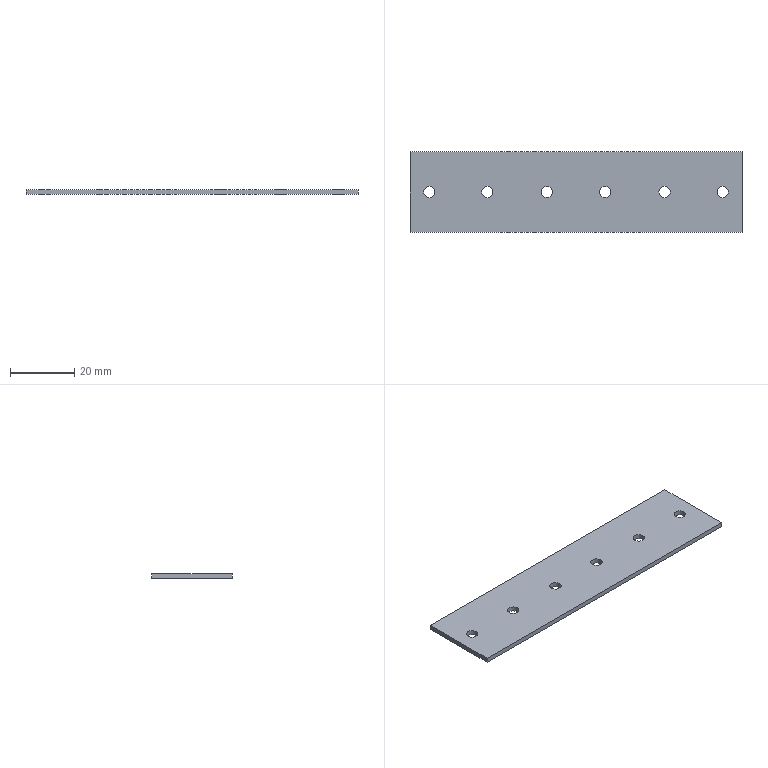Part | STEP file | FHD-021-008-03 fixing plate | 1 solid | 12 faces | box 103 x 25 x 1.5 mm | volume 3776 mm3 | plane 6 | cylinder 6 | commonest cylinder face diameters 3.5 x6
STEP:
#1=CARTESIAN_POINT('',(0.,0.,0.));
#2=DIRECTION('',(0.,0.,1.));
#3=DIRECTION('',(1.,0.,0.));
#4=AXIS2_PLACEMENT_3D('',#1,#2,#3);
#5=CARTESIAN_POINT('',(-51.5,-12.5,-1.5));
#6=VERTEX_POINT('',#5);
#7=CARTESIAN_POINT('',(-51.5,12.5,-1.5));
#8=VERTEX_POINT('',#7);
#9=CARTESIAN_POINT('',(-51.5,0.,-1.5));
#10=DIRECTION('',(0.,1.,0.));
#11=VECTOR('',#10,1.);
#12=LINE('',#9,#11);
#13=CARTESIAN_POINT('',(0.,0.,-1.5));
#14=DIRECTION('',(0.,0.,-1.));
#15=DIRECTION('',(-1.,0.,0.));
#16=AXIS2_PLACEMENT_3D('',#13,#14,#15);
#17=PLANE('',#16);
#18=CARTESIAN_POINT('',(51.5,0.));
#19=DIRECTION('',(0.,1.));
#20=VECTOR('',#19,1.);
#21=LINE('',#18,#20);
#22=(GEOMETRIC_REPRESENTATION_CONTEXT(2)PARAMETRIC_REPRESENTATION_CONTEXT()REPRESENTATION_CONTEXT('',''));
#23=DEFINITIONAL_REPRESENTATION('',(#21),#22);
#24=PCURVE('',#17,#23);
#25=CARTESIAN_POINT('',(-51.5,-12.5,-1.5));
#26=DIRECTION('',(-1.,0.,0.));
#27=DIRECTION('',(0.,0.,1.));
#28=AXIS2_PLACEMENT_3D('',#25,#26,#27);
#29=PLANE('',#28);
#30=CARTESIAN_POINT('',(0.,12.5));
#31=DIRECTION('',(0.,1.));
#32=VECTOR('',#31,1.);
#33=LINE('',#30,#32);
#34=(GEOMETRIC_REPRESENTATION_CONTEXT(2)PARAMETRIC_REPRESENTATION_CONTEXT()REPRESENTATION_CONTEXT('',''));
#35=DEFINITIONAL_REPRESENTATION('',(#33),#34);
#36=PCURVE('',#29,#35);
#37=SURFACE_CURVE('',#12,(#24,#36),.PCURVE_S1.);
#38=EDGE_CURVE('',#6,#8,#37,.T.);
#39=ORIENTED_EDGE('',*,*,#38,.T.);
#40=CARTESIAN_POINT('',(51.5,12.5,-1.5));
#41=VERTEX_POINT('',#40);
#42=CARTESIAN_POINT('',(0.,12.5,-1.5));
#43=DIRECTION('',(1.,0.,0.));
#44=VECTOR('',#43,1.);
#45=LINE('',#42,#44);
#46=CARTESIAN_POINT('',(0.,12.5));
#47=DIRECTION('',(-1.,0.));
#48=VECTOR('',#47,1.);
#49=LINE('',#46,#48);
#50=(GEOMETRIC_REPRESENTATION_CONTEXT(2)PARAMETRIC_REPRESENTATION_CONTEXT()REPRESENTATION_CONTEXT('',''));
#51=DEFINITIONAL_REPRESENTATION('',(#49),#50);
#52=PCURVE('',#17,#51);
#53=CARTESIAN_POINT('',(-51.5,12.5,-1.5));
#54=DIRECTION('',(0.,1.,0.));
#55=DIRECTION('',(0.,0.,1.));
#56=AXIS2_PLACEMENT_3D('',#53,#54,#55);
#57=PLANE('',#56);
#58=CARTESIAN_POINT('',(0.,51.5));
#59=DIRECTION('',(0.,1.));
#60=VECTOR('',#59,1.);
#61=LINE('',#58,#60);
#62=(GEOMETRIC_REPRESENTATION_CONTEXT(2)PARAMETRIC_REPRESENTATION_CONTEXT()REPRESENTATION_CONTEXT('',''));
#63=DEFINITIONAL_REPRESENTATION('',(#61),#62);
#64=PCURVE('',#57,#63);
#65=SURFACE_CURVE('',#45,(#52,#64),.PCURVE_S1.);
#66=EDGE_CURVE('',#8,#41,#65,.T.);
#67=ORIENTED_EDGE('',*,*,#66,.T.);
#68=CARTESIAN_POINT('',(51.5,-12.5,-1.5));
#69=VERTEX_POINT('',#68);
#70=CARTESIAN_POINT('',(51.5,0.,-1.5));
#71=DIRECTION('',(0.,-1.,0.));
#72=VECTOR('',#71,1.);
#73=LINE('',#70,#72);
#74=CARTESIAN_POINT('',(-51.5,0.));
#75=DIRECTION('',(0.,-1.));
#76=VECTOR('',#75,1.);
#77=LINE('',#74,#76);
#78=(GEOMETRIC_REPRESENTATION_CONTEXT(2)PARAMETRIC_REPRESENTATION_CONTEXT()REPRESENTATION_CONTEXT('',''));
#79=DEFINITIONAL_REPRESENTATION('',(#77),#78);
#80=PCURVE('',#17,#79);
#81=CARTESIAN_POINT('',(51.5,-12.5,-1.5));
#82=DIRECTION('',(1.,0.,0.));
#83=DIRECTION('',(0.,0.,-1.));
#84=AXIS2_PLACEMENT_3D('',#81,#82,#83);
#85=PLANE('',#84);
#86=CARTESIAN_POINT('',(0.,12.5));
#87=DIRECTION('',(0.,-1.));
#88=VECTOR('',#87,1.);
#89=LINE('',#86,#88);
#90=(GEOMETRIC_REPRESENTATION_CONTEXT(2)PARAMETRIC_REPRESENTATION_CONTEXT()REPRESENTATION_CONTEXT('',''));
#91=DEFINITIONAL_REPRESENTATION('',(#89),#90);
#92=PCURVE('',#85,#91);
#93=SURFACE_CURVE('',#73,(#80,#92),.PCURVE_S1.);
#94=EDGE_CURVE('',#41,#69,#93,.T.);
#95=ORIENTED_EDGE('',*,*,#94,.T.);
#96=CARTESIAN_POINT('',(0.,-12.5,-1.5));
#97=DIRECTION('',(-1.,0.,0.));
#98=VECTOR('',#97,1.);
#99=LINE('',#96,#98);
#100=CARTESIAN_POINT('',(0.,-12.5));
#101=DIRECTION('',(1.,0.));
#102=VECTOR('',#101,1.);
#103=LINE('',#100,#102);
#104=(GEOMETRIC_REPRESENTATION_CONTEXT(2)PARAMETRIC_REPRESENTATION_CONTEXT()REPRESENTATION_CONTEXT('',''));
#105=DEFINITIONAL_REPRESENTATION('',(#103),#104);
#106=PCURVE('',#17,#105);
#107=CARTESIAN_POINT('',(-51.5,-12.5,-1.5));
#108=DIRECTION('',(0.,-1.,0.));
#109=DIRECTION('',(0.,0.,-1.));
#110=AXIS2_PLACEMENT_3D('',#107,#108,#109);
#111=PLANE('',#110);
#112=CARTESIAN_POINT('',(0.,51.5));
#113=DIRECTION('',(0.,-1.));
#114=VECTOR('',#113,1.);
#115=LINE('',#112,#114);
#116=(GEOMETRIC_REPRESENTATION_CONTEXT(2)PARAMETRIC_REPRESENTATION_CONTEXT()REPRESENTATION_CONTEXT('',''));
#117=DEFINITIONAL_REPRESENTATION('',(#115),#116);
#118=PCURVE('',#111,#117);
#119=SURFACE_CURVE('',#99,(#106,#118),.PCURVE_S1.);
#120=EDGE_CURVE('',#69,#6,#119,.T.);
#121=ORIENTED_EDGE('',*,*,#120,.T.);
#122=EDGE_LOOP('',(#39,#67,#95,#121));
#123=FACE_BOUND('',#122,.T.);
#124=CARTESIAN_POINT('',(47.25,0.,-1.5));
#125=VERTEX_POINT('',#124);
#126=CARTESIAN_POINT('',(45.5,0.,-1.5));
#127=DIRECTION('',(0.,0.,1.));
#128=DIRECTION('',(1.,0.,0.));
#129=AXIS2_PLACEMENT_3D('',#126,#127,#128);
#130=CIRCLE('',#129,1.75);
#131=CARTESIAN_POINT('',(-47.25,0.));
#132=CARTESIAN_POINT('',(-47.25,3.031));
#133=CARTESIAN_POINT('',(-44.625,1.516));
#134=CARTESIAN_POINT('',(-42.,0.));
#135=CARTESIAN_POINT('',(-44.625,-1.516));
#136=CARTESIAN_POINT('',(-47.25,-3.031));
#137=CARTESIAN_POINT('',(-47.25,0.));
#138=(BOUNDED_CURVE()B_SPLINE_CURVE(2,(#131,#132,#133,#134,#135,#136,#137),.UNSPECIFIED.,.T.,.F.)B_SPLINE_CURVE_WITH_KNOTS((1,2,2,2,2,1),(-2.094,0.,2.094,4.189,6.283,8.378),.UNSPECIFIED.)CURVE()GEOMETRIC_REPRESENTATION_ITEM()RATIONAL_B_SPLINE_CURVE((1.,0.5,1.,0.5,1.,0.5,1.))REPRESENTATION_ITEM(''));
#139=(GEOMETRIC_REPRESENTATION_CONTEXT(2)PARAMETRIC_REPRESENTATION_CONTEXT()REPRESENTATION_CONTEXT('',''));
#140=DEFINITIONAL_REPRESENTATION('',(#138),#139);
#141=PCURVE('',#17,#140);
#142=CARTESIAN_POINT('',(45.5,0.,-10.));
#143=DIRECTION('',(0.,0.,1.));
#144=DIRECTION('',(1.,0.,0.));
#145=AXIS2_PLACEMENT_3D('',#142,#143,#144);
#146=CYLINDRICAL_SURFACE('',#145,1.75);
#147=CARTESIAN_POINT('',(0.,8.5));
#148=DIRECTION('',(1.,0.));
#149=VECTOR('',#148,1.);
#150=LINE('',#147,#149);
#151=(GEOMETRIC_REPRESENTATION_CONTEXT(2)PARAMETRIC_REPRESENTATION_CONTEXT()REPRESENTATION_CONTEXT('',''));
#152=DEFINITIONAL_REPRESENTATION('',(#150),#151);
#153=PCURVE('',#146,#152);
#154=SURFACE_CURVE('',#130,(#141,#153),.PCURVE_S1.);
#155=EDGE_CURVE('',#125,#125,#154,.T.);
#156=ORIENTED_EDGE('',*,*,#155,.T.);
#157=EDGE_LOOP('',(#156));
#158=FACE_BOUND('',#157,.T.);
#159=CARTESIAN_POINT('',(-43.75,0.,-1.5));
#160=VERTEX_POINT('',#159);
#161=CARTESIAN_POINT('',(-45.5,0.,-1.5));
#162=DIRECTION('',(0.,0.,1.));
#163=DIRECTION('',(1.,0.,0.));
#164=AXIS2_PLACEMENT_3D('',#161,#162,#163);
#165=CIRCLE('',#164,1.75);
#166=CARTESIAN_POINT('',(43.75,0.));
#167=CARTESIAN_POINT('',(43.75,3.031));
#168=CARTESIAN_POINT('',(46.375,1.516));
#169=CARTESIAN_POINT('',(49.,0.));
#170=CARTESIAN_POINT('',(46.375,-1.516));
#171=CARTESIAN_POINT('',(43.75,-3.031));
#172=CARTESIAN_POINT('',(43.75,0.));
#173=(BOUNDED_CURVE()B_SPLINE_CURVE(2,(#166,#167,#168,#169,#170,#171,#172),.UNSPECIFIED.,.T.,.F.)B_SPLINE_CURVE_WITH_KNOTS((1,2,2,2,2,1),(-2.094,0.,2.094,4.189,6.283,8.378),.UNSPECIFIED.)CURVE()GEOMETRIC_REPRESENTATION_ITEM()RATIONAL_B_SPLINE_CURVE((1.,0.5,1.,0.5,1.,0.5,1.))REPRESENTATION_ITEM(''));
#174=(GEOMETRIC_REPRESENTATION_CONTEXT(2)PARAMETRIC_REPRESENTATION_CONTEXT()REPRESENTATION_CONTEXT('',''));
#175=DEFINITIONAL_REPRESENTATION('',(#173),#174);
#176=PCURVE('',#17,#175);
#177=CARTESIAN_POINT('',(-45.5,0.,-10.));
#178=DIRECTION('',(0.,0.,1.));
#179=DIRECTION('',(1.,0.,0.));
#180=AXIS2_PLACEMENT_3D('',#177,#178,#179);
#181=CYLINDRICAL_SURFACE('',#180,1.75);
#182=CARTESIAN_POINT('',(0.,8.5));
#183=DIRECTION('',(1.,0.));
#184=VECTOR('',#183,1.);
#185=LINE('',#182,#184);
#186=(GEOMETRIC_REPRESENTATION_CONTEXT(2)PARAMETRIC_REPRESENTATION_CONTEXT()REPRESENTATION_CONTEXT('',''));
#187=DEFINITIONAL_REPRESENTATION('',(#185),#186);
#188=PCURVE('',#181,#187);
#189=SURFACE_CURVE('',#165,(#176,#188),.PCURVE_S1.);
#190=EDGE_CURVE('',#160,#160,#189,.T.);
#191=ORIENTED_EDGE('',*,*,#190,.T.);
#192=EDGE_LOOP('',(#191));
#193=FACE_BOUND('',#192,.T.);
#194=CARTESIAN_POINT('',(29.25,0.,-1.5));
#195=VERTEX_POINT('',#194);
#196=CARTESIAN_POINT('',(27.5,0.,-1.5));
#197=DIRECTION('',(0.,0.,1.));
#198=DIRECTION('',(1.,0.,0.));
#199=AXIS2_PLACEMENT_3D('',#196,#197,#198);
#200=CIRCLE('',#199,1.75);
#201=CARTESIAN_POINT('',(-29.25,0.));
#202=CARTESIAN_POINT('',(-29.25,3.031));
#203=CARTESIAN_POINT('',(-26.625,1.516));
#204=CARTESIAN_POINT('',(-24.,0.));
#205=CARTESIAN_POINT('',(-26.625,-1.516));
#206=CARTESIAN_POINT('',(-29.25,-3.031));
#207=CARTESIAN_POINT('',(-29.25,0.));
#208=(BOUNDED_CURVE()B_SPLINE_CURVE(2,(#201,#202,#203,#204,#205,#206,#207),.UNSPECIFIED.,.T.,.F.)B_SPLINE_CURVE_WITH_KNOTS((1,2,2,2,2,1),(-2.094,0.,2.094,4.189,6.283,8.378),.UNSPECIFIED.)CURVE()GEOMETRIC_REPRESENTATION_ITEM()RATIONAL_B_SPLINE_CURVE((1.,0.5,1.,0.5,1.,0.5,1.))REPRESENTATION_ITEM(''));
#209=(GEOMETRIC_REPRESENTATION_CONTEXT(2)PARAMETRIC_REPRESENTATION_CONTEXT()REPRESENTATION_CONTEXT('',''));
#210=DEFINITIONAL_REPRESENTATION('',(#208),#209);
#211=PCURVE('',#17,#210);
#212=CARTESIAN_POINT('',(27.5,0.,-10.));
#213=DIRECTION('',(0.,0.,1.));
#214=DIRECTION('',(1.,0.,0.));
#215=AXIS2_PLACEMENT_3D('',#212,#213,#214);
#216=CYLINDRICAL_SURFACE('',#215,1.75);
#217=CARTESIAN_POINT('',(0.,8.5));
#218=DIRECTION('',(1.,0.));
#219=VECTOR('',#218,1.);
#220=LINE('',#217,#219);
#221=(GEOMETRIC_REPRESENTATION_CONTEXT(2)PARAMETRIC_REPRESENTATION_CONTEXT()REPRESENTATION_CONTEXT('',''));
#222=DEFINITIONAL_REPRESENTATION('',(#220),#221);
#223=PCURVE('',#216,#222);
#224=SURFACE_CURVE('',#200,(#211,#223),.PCURVE_S1.);
#225=EDGE_CURVE('',#195,#195,#224,.T.);
#226=ORIENTED_EDGE('',*,*,#225,.T.);
#227=EDGE_LOOP('',(#226));
#228=FACE_BOUND('',#227,.T.);
#229=CARTESIAN_POINT('',(10.75,0.,-1.5));
#230=VERTEX_POINT('',#229);
#231=CARTESIAN_POINT('',(9.,0.,-1.5));
#232=DIRECTION('',(0.,0.,1.));
#233=DIRECTION('',(1.,0.,0.));
#234=AXIS2_PLACEMENT_3D('',#231,#232,#233);
#235=CIRCLE('',#234,1.75);
#236=CARTESIAN_POINT('',(-10.75,0.));
#237=CARTESIAN_POINT('',(-10.75,3.031));
#238=CARTESIAN_POINT('',(-8.125,1.516));
#239=CARTESIAN_POINT('',(-5.5,0.));
#240=CARTESIAN_POINT('',(-8.125,-1.516));
#241=CARTESIAN_POINT('',(-10.75,-3.031));
#242=CARTESIAN_POINT('',(-10.75,0.));
#243=(BOUNDED_CURVE()B_SPLINE_CURVE(2,(#236,#237,#238,#239,#240,#241,#242),.UNSPECIFIED.,.T.,.F.)B_SPLINE_CURVE_WITH_KNOTS((1,2,2,2,2,1),(-2.094,0.,2.094,4.189,6.283,8.378),.UNSPECIFIED.)CURVE()GEOMETRIC_REPRESENTATION_ITEM()RATIONAL_B_SPLINE_CURVE((1.,0.5,1.,0.5,1.,0.5,1.))REPRESENTATION_ITEM(''));
#244=(GEOMETRIC_REPRESENTATION_CONTEXT(2)PARAMETRIC_REPRESENTATION_CONTEXT()REPRESENTATION_CONTEXT('',''));
#245=DEFINITIONAL_REPRESENTATION('',(#243),#244);
#246=PCURVE('',#17,#245);
#247=CARTESIAN_POINT('',(9.,0.,-10.));
#248=DIRECTION('',(0.,0.,1.));
#249=DIRECTION('',(1.,0.,0.));
#250=AXIS2_PLACEMENT_3D('',#247,#248,#249);
#251=CYLINDRICAL_SURFACE('',#250,1.75);
#252=CARTESIAN_POINT('',(0.,8.5));
#253=DIRECTION('',(1.,0.));
#254=VECTOR('',#253,1.);
#255=LINE('',#252,#254);
#256=(GEOMETRIC_REPRESENTATION_CONTEXT(2)PARAMETRIC_REPRESENTATION_CONTEXT()REPRESENTATION_CONTEXT('',''));
#257=DEFINITIONAL_REPRESENTATION('',(#255),#256);
#258=PCURVE('',#251,#257);
#259=SURFACE_CURVE('',#235,(#246,#258),.PCURVE_S1.);
#260=EDGE_CURVE('',#230,#230,#259,.T.);
#261=ORIENTED_EDGE('',*,*,#260,.T.);
#262=EDGE_LOOP('',(#261));
#263=FACE_BOUND('',#262,.T.);
#264=CARTESIAN_POINT('',(-7.25,0.,-1.5));
#265=VERTEX_POINT('',#264);
#266=CARTESIAN_POINT('',(-9.,0.,-1.5));
#267=DIRECTION('',(0.,0.,1.));
#268=DIRECTION('',(1.,0.,0.));
#269=AXIS2_PLACEMENT_3D('',#266,#267,#268);
#270=CIRCLE('',#269,1.75);
#271=CARTESIAN_POINT('',(7.25,0.));
#272=CARTESIAN_POINT('',(7.25,3.031));
#273=CARTESIAN_POINT('',(9.875,1.516));
#274=CARTESIAN_POINT('',(12.5,0.));
#275=CARTESIAN_POINT('',(9.875,-1.516));
#276=CARTESIAN_POINT('',(7.25,-3.031));
#277=CARTESIAN_POINT('',(7.25,0.));
#278=(BOUNDED_CURVE()B_SPLINE_CURVE(2,(#271,#272,#273,#274,#275,#276,#277),.UNSPECIFIED.,.T.,.F.)B_SPLINE_CURVE_WITH_KNOTS((1,2,2,2,2,1),(-2.094,0.,2.094,4.189,6.283,8.378),.UNSPECIFIED.)CURVE()GEOMETRIC_REPRESENTATION_ITEM()RATIONAL_B_SPLINE_CURVE((1.,0.5,1.,0.5,1.,0.5,1.))REPRESENTATION_ITEM(''));
#279=(GEOMETRIC_REPRESENTATION_CONTEXT(2)PARAMETRIC_REPRESENTATION_CONTEXT()REPRESENTATION_CONTEXT('',''));
#280=DEFINITIONAL_REPRESENTATION('',(#278),#279);
#281=PCURVE('',#17,#280);
#282=CARTESIAN_POINT('',(-9.,0.,-10.));
#283=DIRECTION('',(0.,0.,1.));
#284=DIRECTION('',(1.,0.,0.));
#285=AXIS2_PLACEMENT_3D('',#282,#283,#284);
#286=CYLINDRICAL_SURFACE('',#285,1.75);
#287=CARTESIAN_POINT('',(0.,8.5));
#288=DIRECTION('',(1.,0.));
#289=VECTOR('',#288,1.);
#290=LINE('',#287,#289);
#291=(GEOMETRIC_REPRESENTATION_CONTEXT(2)PARAMETRIC_REPRESENTATION_CONTEXT()REPRESENTATION_CONTEXT('',''));
#292=DEFINITIONAL_REPRESENTATION('',(#290),#291);
#293=PCURVE('',#286,#292);
#294=SURFACE_CURVE('',#270,(#281,#293),.PCURVE_S1.);
#295=EDGE_CURVE('',#265,#265,#294,.T.);
#296=ORIENTED_EDGE('',*,*,#295,.T.);
#297=EDGE_LOOP('',(#296));
#298=FACE_BOUND('',#297,.T.);
#299=CARTESIAN_POINT('',(-25.75,0.,-1.5));
#300=VERTEX_POINT('',#299);
#301=CARTESIAN_POINT('',(-27.5,0.,-1.5));
#302=DIRECTION('',(0.,0.,1.));
#303=DIRECTION('',(1.,0.,0.));
#304=AXIS2_PLACEMENT_3D('',#301,#302,#303);
#305=CIRCLE('',#304,1.75);
#306=CARTESIAN_POINT('',(25.75,0.));
#307=CARTESIAN_POINT('',(25.75,3.031));
#308=CARTESIAN_POINT('',(28.375,1.516));
#309=CARTESIAN_POINT('',(31.,0.));
#310=CARTESIAN_POINT('',(28.375,-1.516));
#311=CARTESIAN_POINT('',(25.75,-3.031));
#312=CARTESIAN_POINT('',(25.75,0.));
#313=(BOUNDED_CURVE()B_SPLINE_CURVE(2,(#306,#307,#308,#309,#310,#311,#312),.UNSPECIFIED.,.T.,.F.)B_SPLINE_CURVE_WITH_KNOTS((1,2,2,2,2,1),(-2.094,0.,2.094,4.189,6.283,8.378),.UNSPECIFIED.)CURVE()GEOMETRIC_REPRESENTATION_ITEM()RATIONAL_B_SPLINE_CURVE((1.,0.5,1.,0.5,1.,0.5,1.))REPRESENTATION_ITEM(''));
#314=(GEOMETRIC_REPRESENTATION_CONTEXT(2)PARAMETRIC_REPRESENTATION_CONTEXT()REPRESENTATION_CONTEXT('',''));
#315=DEFINITIONAL_REPRESENTATION('',(#313),#314);
#316=PCURVE('',#17,#315);
#317=CARTESIAN_POINT('',(-27.5,0.,-10.));
#318=DIRECTION('',(0.,0.,1.));
#319=DIRECTION('',(1.,0.,0.));
#320=AXIS2_PLACEMENT_3D('',#317,#318,#319);
#321=CYLINDRICAL_SURFACE('',#320,1.75);
#322=CARTESIAN_POINT('',(0.,8.5));
#323=DIRECTION('',(1.,0.));
#324=VECTOR('',#323,1.);
#325=LINE('',#322,#324);
#326=(GEOMETRIC_REPRESENTATION_CONTEXT(2)PARAMETRIC_REPRESENTATION_CONTEXT()REPRESENTATION_CONTEXT('',''));
#327=DEFINITIONAL_REPRESENTATION('',(#325),#326);
#328=PCURVE('',#321,#327);
#329=SURFACE_CURVE('',#305,(#316,#328),.PCURVE_S1.);
#330=EDGE_CURVE('',#300,#300,#329,.T.);
#331=ORIENTED_EDGE('',*,*,#330,.T.);
#332=EDGE_LOOP('',(#331));
#333=FACE_BOUND('',#332,.T.);
#334=ADVANCED_FACE('',(#123,#158,#193,#228,#263,#298,#333),#17,.T.);
#335=ORIENTED_EDGE('',*,*,#66,.F.);
#336=CARTESIAN_POINT('',(-51.5,12.5,0.));
#337=VERTEX_POINT('',#336);
#338=CARTESIAN_POINT('',(-51.5,12.5,-1.5));
#339=DIRECTION('',(0.,0.,1.));
#340=VECTOR('',#339,1.);
#341=LINE('',#338,#340);
#342=CARTESIAN_POINT('',(0.,0.));
#343=DIRECTION('',(1.,0.));
#344=VECTOR('',#343,1.);
#345=LINE('',#342,#344);
#346=(GEOMETRIC_REPRESENTATION_CONTEXT(2)PARAMETRIC_REPRESENTATION_CONTEXT()REPRESENTATION_CONTEXT('',''));
#347=DEFINITIONAL_REPRESENTATION('',(#345),#346);
#348=PCURVE('',#57,#347);
#349=CARTESIAN_POINT('',(0.,25.));
#350=DIRECTION('',(1.,0.));
#351=VECTOR('',#350,1.);
#352=LINE('',#349,#351);
#353=(GEOMETRIC_REPRESENTATION_CONTEXT(2)PARAMETRIC_REPRESENTATION_CONTEXT()REPRESENTATION_CONTEXT('',''));
#354=DEFINITIONAL_REPRESENTATION('',(#352),#353);
#355=PCURVE('',#29,#354);
#356=SURFACE_CURVE('',#341,(#348,#355),.PCURVE_S1.);
#357=EDGE_CURVE('',#8,#337,#356,.T.);
#358=ORIENTED_EDGE('',*,*,#357,.T.);
#359=CARTESIAN_POINT('',(51.5,12.5,0.));
#360=VERTEX_POINT('',#359);
#361=CARTESIAN_POINT('',(-51.5,12.5,0.));
#362=DIRECTION('',(1.,0.,0.));
#363=VECTOR('',#362,1.);
#364=LINE('',#361,#363);
#365=CARTESIAN_POINT('',(1.5,0.));
#366=DIRECTION('',(0.,1.));
#367=VECTOR('',#366,1.);
#368=LINE('',#365,#367);
#369=(GEOMETRIC_REPRESENTATION_CONTEXT(2)PARAMETRIC_REPRESENTATION_CONTEXT()REPRESENTATION_CONTEXT('',''));
#370=DEFINITIONAL_REPRESENTATION('',(#368),#369);
#371=PCURVE('',#57,#370);
#372=CARTESIAN_POINT('',(0.,0.,0.));
#373=DIRECTION('',(0.,0.,-1.));
#374=DIRECTION('',(-1.,0.,0.));
#375=AXIS2_PLACEMENT_3D('',#372,#373,#374);
#376=PLANE('',#375);
#377=CARTESIAN_POINT('',(51.5,12.5));
#378=DIRECTION('',(-1.,0.));
#379=VECTOR('',#378,1.);
#380=LINE('',#377,#379);
#381=(GEOMETRIC_REPRESENTATION_CONTEXT(2)PARAMETRIC_REPRESENTATION_CONTEXT()REPRESENTATION_CONTEXT('',''));
#382=DEFINITIONAL_REPRESENTATION('',(#380),#381);
#383=PCURVE('',#376,#382);
#384=SURFACE_CURVE('',#364,(#371,#383),.PCURVE_S1.);
#385=EDGE_CURVE('',#337,#360,#384,.T.);
#386=ORIENTED_EDGE('',*,*,#385,.T.);
#387=CARTESIAN_POINT('',(51.5,12.5,-1.5));
#388=DIRECTION('',(0.,0.,-1.));
#389=VECTOR('',#388,1.);
#390=LINE('',#387,#389);
#391=CARTESIAN_POINT('',(0.,103.));
#392=DIRECTION('',(-1.,0.));
#393=VECTOR('',#392,1.);
#394=LINE('',#391,#393);
#395=(GEOMETRIC_REPRESENTATION_CONTEXT(2)PARAMETRIC_REPRESENTATION_CONTEXT()REPRESENTATION_CONTEXT('',''));
#396=DEFINITIONAL_REPRESENTATION('',(#394),#395);
#397=PCURVE('',#57,#396);
#398=CARTESIAN_POINT('',(0.,25.));
#399=DIRECTION('',(1.,0.));
#400=VECTOR('',#399,1.);
#401=LINE('',#398,#400);
#402=(GEOMETRIC_REPRESENTATION_CONTEXT(2)PARAMETRIC_REPRESENTATION_CONTEXT()REPRESENTATION_CONTEXT('',''));
#403=DEFINITIONAL_REPRESENTATION('',(#401),#402);
#404=PCURVE('',#85,#403);
#405=SURFACE_CURVE('',#390,(#397,#404),.PCURVE_S1.);
#406=EDGE_CURVE('',#360,#41,#405,.T.);
#407=ORIENTED_EDGE('',*,*,#406,.T.);
#408=EDGE_LOOP('',(#335,#358,#386,#407));
#409=FACE_BOUND('',#408,.T.);
#410=ADVANCED_FACE('',(#409),#57,.T.);
#411=ORIENTED_EDGE('',*,*,#38,.F.);
#412=CARTESIAN_POINT('',(-51.5,-12.5,0.));
#413=VERTEX_POINT('',#412);
#414=CARTESIAN_POINT('',(-51.5,-12.5,-1.5));
#415=DIRECTION('',(0.,0.,1.));
#416=VECTOR('',#415,1.);
#417=LINE('',#414,#416);
#418=CARTESIAN_POINT('',(0.,0.));
#419=DIRECTION('',(1.,0.));
#420=VECTOR('',#419,1.);
#421=LINE('',#418,#420);
#422=(GEOMETRIC_REPRESENTATION_CONTEXT(2)PARAMETRIC_REPRESENTATION_CONTEXT()REPRESENTATION_CONTEXT('',''));
#423=DEFINITIONAL_REPRESENTATION('',(#421),#422);
#424=PCURVE('',#29,#423);
#425=CARTESIAN_POINT('',(0.,0.));
#426=DIRECTION('',(-1.,0.));
#427=VECTOR('',#426,1.);
#428=LINE('',#425,#427);
#429=(GEOMETRIC_REPRESENTATION_CONTEXT(2)PARAMETRIC_REPRESENTATION_CONTEXT()REPRESENTATION_CONTEXT('',''));
#430=DEFINITIONAL_REPRESENTATION('',(#428),#429);
#431=PCURVE('',#111,#430);
#432=SURFACE_CURVE('',#417,(#424,#431),.PCURVE_S1.);
#433=EDGE_CURVE('',#6,#413,#432,.T.);
#434=ORIENTED_EDGE('',*,*,#433,.T.);
#435=CARTESIAN_POINT('',(-51.5,-12.5,0.));
#436=DIRECTION('',(0.,1.,0.));
#437=VECTOR('',#436,1.);
#438=LINE('',#435,#437);
#439=CARTESIAN_POINT('',(1.5,0.));
#440=DIRECTION('',(0.,1.));
#441=VECTOR('',#440,1.);
#442=LINE('',#439,#441);
#443=(GEOMETRIC_REPRESENTATION_CONTEXT(2)PARAMETRIC_REPRESENTATION_CONTEXT()REPRESENTATION_CONTEXT('',''));
#444=DEFINITIONAL_REPRESENTATION('',(#442),#443);
#445=PCURVE('',#29,#444);
#446=CARTESIAN_POINT('',(51.5,-12.5));
#447=DIRECTION('',(0.,1.));
#448=VECTOR('',#447,1.);
#449=LINE('',#446,#448);
#450=(GEOMETRIC_REPRESENTATION_CONTEXT(2)PARAMETRIC_REPRESENTATION_CONTEXT()REPRESENTATION_CONTEXT('',''));
#451=DEFINITIONAL_REPRESENTATION('',(#449),#450);
#452=PCURVE('',#376,#451);
#453=SURFACE_CURVE('',#438,(#445,#452),.PCURVE_S1.);
#454=EDGE_CURVE('',#413,#337,#453,.T.);
#455=ORIENTED_EDGE('',*,*,#454,.T.);
#456=ORIENTED_EDGE('',*,*,#357,.F.);
#457=EDGE_LOOP('',(#411,#434,#455,#456));
#458=FACE_BOUND('',#457,.T.);
#459=ADVANCED_FACE('',(#458),#29,.T.);
#460=ORIENTED_EDGE('',*,*,#120,.F.);
#461=CARTESIAN_POINT('',(51.5,-12.5,0.));
#462=VERTEX_POINT('',#461);
#463=CARTESIAN_POINT('',(51.5,-12.5,-1.5));
#464=DIRECTION('',(0.,0.,1.));
#465=VECTOR('',#464,1.);
#466=LINE('',#463,#465);
#467=CARTESIAN_POINT('',(0.,103.));
#468=DIRECTION('',(-1.,0.));
#469=VECTOR('',#468,1.);
#470=LINE('',#467,#469);
#471=(GEOMETRIC_REPRESENTATION_CONTEXT(2)PARAMETRIC_REPRESENTATION_CONTEXT()REPRESENTATION_CONTEXT('',''));
#472=DEFINITIONAL_REPRESENTATION('',(#470),#471);
#473=PCURVE('',#111,#472);
#474=CARTESIAN_POINT('',(0.,0.));
#475=DIRECTION('',(-1.,0.));
#476=VECTOR('',#475,1.);
#477=LINE('',#474,#476);
#478=(GEOMETRIC_REPRESENTATION_CONTEXT(2)PARAMETRIC_REPRESENTATION_CONTEXT()REPRESENTATION_CONTEXT('',''));
#479=DEFINITIONAL_REPRESENTATION('',(#477),#478);
#480=PCURVE('',#85,#479);
#481=SURFACE_CURVE('',#466,(#473,#480),.PCURVE_S1.);
#482=EDGE_CURVE('',#69,#462,#481,.T.);
#483=ORIENTED_EDGE('',*,*,#482,.T.);
#484=CARTESIAN_POINT('',(-51.5,-12.5,0.));
#485=DIRECTION('',(-1.,0.,0.));
#486=VECTOR('',#485,1.);
#487=LINE('',#484,#486);
#488=CARTESIAN_POINT('',(-1.5,0.));
#489=DIRECTION('',(0.,-1.));
#490=VECTOR('',#489,1.);
#491=LINE('',#488,#490);
#492=(GEOMETRIC_REPRESENTATION_CONTEXT(2)PARAMETRIC_REPRESENTATION_CONTEXT()REPRESENTATION_CONTEXT('',''));
#493=DEFINITIONAL_REPRESENTATION('',(#491),#492);
#494=PCURVE('',#111,#493);
#495=CARTESIAN_POINT('',(51.5,-12.5));
#496=DIRECTION('',(1.,0.));
#497=VECTOR('',#496,1.);
#498=LINE('',#495,#497);
#499=(GEOMETRIC_REPRESENTATION_CONTEXT(2)PARAMETRIC_REPRESENTATION_CONTEXT()REPRESENTATION_CONTEXT('',''));
#500=DEFINITIONAL_REPRESENTATION('',(#498),#499);
#501=PCURVE('',#376,#500);
#502=SURFACE_CURVE('',#487,(#494,#501),.PCURVE_S1.);
#503=EDGE_CURVE('',#462,#413,#502,.T.);
#504=ORIENTED_EDGE('',*,*,#503,.T.);
#505=ORIENTED_EDGE('',*,*,#433,.F.);
#506=EDGE_LOOP('',(#460,#483,#504,#505));
#507=FACE_BOUND('',#506,.T.);
#508=ADVANCED_FACE('',(#507),#111,.T.);
#509=ORIENTED_EDGE('',*,*,#94,.F.);
#510=ORIENTED_EDGE('',*,*,#406,.F.);
#511=CARTESIAN_POINT('',(51.5,-12.5,0.));
#512=DIRECTION('',(0.,-1.,0.));
#513=VECTOR('',#512,1.);
#514=LINE('',#511,#513);
#515=CARTESIAN_POINT('',(-1.5,0.));
#516=DIRECTION('',(0.,-1.));
#517=VECTOR('',#516,1.);
#518=LINE('',#515,#517);
#519=(GEOMETRIC_REPRESENTATION_CONTEXT(2)PARAMETRIC_REPRESENTATION_CONTEXT()REPRESENTATION_CONTEXT('',''));
#520=DEFINITIONAL_REPRESENTATION('',(#518),#519);
#521=PCURVE('',#85,#520);
#522=CARTESIAN_POINT('',(-51.5,-12.5));
#523=DIRECTION('',(0.,-1.));
#524=VECTOR('',#523,1.);
#525=LINE('',#522,#524);
#526=(GEOMETRIC_REPRESENTATION_CONTEXT(2)PARAMETRIC_REPRESENTATION_CONTEXT()REPRESENTATION_CONTEXT('',''));
#527=DEFINITIONAL_REPRESENTATION('',(#525),#526);
#528=PCURVE('',#376,#527);
#529=SURFACE_CURVE('',#514,(#521,#528),.PCURVE_S1.);
#530=EDGE_CURVE('',#360,#462,#529,.T.);
#531=ORIENTED_EDGE('',*,*,#530,.T.);
#532=ORIENTED_EDGE('',*,*,#482,.F.);
#533=EDGE_LOOP('',(#509,#510,#531,#532));
#534=FACE_BOUND('',#533,.T.);
#535=ADVANCED_FACE('',(#534),#85,.T.);
#536=ORIENTED_EDGE('',*,*,#155,.T.);
#537=CARTESIAN_POINT('',(47.25,0.,0.));
#538=VERTEX_POINT('',#537);
#539=CARTESIAN_POINT('',(47.25,0.,-1.5));
#540=CARTESIAN_POINT('',(47.25,0.,0.));
#541=B_SPLINE_CURVE_WITH_KNOTS('',1,(#539,#540),.UNSPECIFIED.,.F.,.F.,(2,2),(8.5,10.),.PIECEWISE_BEZIER_KNOTS.);
#542=CARTESIAN_POINT('',(6.283,0.));
#543=DIRECTION('',(0.,1.));
#544=VECTOR('',#543,1.);
#545=LINE('',#542,#544);
#546=(GEOMETRIC_REPRESENTATION_CONTEXT(2)PARAMETRIC_REPRESENTATION_CONTEXT()REPRESENTATION_CONTEXT('',''));
#547=DEFINITIONAL_REPRESENTATION('',(#545),#546);
#548=PCURVE('',#146,#547);
#549=CARTESIAN_POINT('',(0.,0.));
#550=DIRECTION('',(0.,1.));
#551=VECTOR('',#550,1.);
#552=LINE('',#549,#551);
#553=(GEOMETRIC_REPRESENTATION_CONTEXT(2)PARAMETRIC_REPRESENTATION_CONTEXT()REPRESENTATION_CONTEXT('',''));
#554=DEFINITIONAL_REPRESENTATION('',(#552),#553);
#555=PCURVE('',#146,#554);
#556=SEAM_CURVE('',#541,(#548,#555),.PCURVE_S1.);
#557=EDGE_CURVE('',#125,#538,#556,.T.);
#558=ORIENTED_EDGE('',*,*,#557,.T.);
#559=CARTESIAN_POINT('',(45.5,0.,0.));
#560=DIRECTION('',(0.,0.,-1.));
#561=DIRECTION('',(1.,0.,0.));
#562=AXIS2_PLACEMENT_3D('',#559,#560,#561);
#563=CIRCLE('',#562,1.75);
#564=CARTESIAN_POINT('',(6.283,10.));
#565=DIRECTION('',(-1.,0.));
#566=VECTOR('',#565,1.);
#567=LINE('',#564,#566);
#568=(GEOMETRIC_REPRESENTATION_CONTEXT(2)PARAMETRIC_REPRESENTATION_CONTEXT()REPRESENTATION_CONTEXT('',''));
#569=DEFINITIONAL_REPRESENTATION('',(#567),#568);
#570=PCURVE('',#146,#569);
#571=CARTESIAN_POINT('',(-45.5,0.));
#572=DIRECTION('',(-1.,0.));
#573=AXIS2_PLACEMENT_2D('',#571,#572);
#574=CIRCLE('',#573,1.75);
#575=(GEOMETRIC_REPRESENTATION_CONTEXT(2)PARAMETRIC_REPRESENTATION_CONTEXT()REPRESENTATION_CONTEXT('',''));
#576=DEFINITIONAL_REPRESENTATION('',(#574),#575);
#577=PCURVE('',#376,#576);
#578=SURFACE_CURVE('',#563,(#570,#577),.PCURVE_S1.);
#579=EDGE_CURVE('',#538,#538,#578,.T.);
#580=ORIENTED_EDGE('',*,*,#579,.T.);
#581=ORIENTED_EDGE('',*,*,#557,.F.);
#582=EDGE_LOOP('',(#536,#558,#580,#581));
#583=FACE_BOUND('',#582,.F.);
#584=ADVANCED_FACE('',(#583),#146,.F.);
#585=ORIENTED_EDGE('',*,*,#190,.T.);
#586=CARTESIAN_POINT('',(-43.75,0.,0.));
#587=VERTEX_POINT('',#586);
#588=CARTESIAN_POINT('',(-43.75,0.,-1.5));
#589=CARTESIAN_POINT('',(-43.75,0.,0.));
#590=B_SPLINE_CURVE_WITH_KNOTS('',1,(#588,#589),.UNSPECIFIED.,.F.,.F.,(2,2),(8.5,10.),.PIECEWISE_BEZIER_KNOTS.);
#591=CARTESIAN_POINT('',(6.283,0.));
#592=DIRECTION('',(0.,1.));
#593=VECTOR('',#592,1.);
#594=LINE('',#591,#593);
#595=(GEOMETRIC_REPRESENTATION_CONTEXT(2)PARAMETRIC_REPRESENTATION_CONTEXT()REPRESENTATION_CONTEXT('',''));
#596=DEFINITIONAL_REPRESENTATION('',(#594),#595);
#597=PCURVE('',#181,#596);
#598=CARTESIAN_POINT('',(0.,0.));
#599=DIRECTION('',(0.,1.));
#600=VECTOR('',#599,1.);
#601=LINE('',#598,#600);
#602=(GEOMETRIC_REPRESENTATION_CONTEXT(2)PARAMETRIC_REPRESENTATION_CONTEXT()REPRESENTATION_CONTEXT('',''));
#603=DEFINITIONAL_REPRESENTATION('',(#601),#602);
#604=PCURVE('',#181,#603);
#605=SEAM_CURVE('',#590,(#597,#604),.PCURVE_S1.);
#606=EDGE_CURVE('',#160,#587,#605,.T.);
#607=ORIENTED_EDGE('',*,*,#606,.T.);
#608=CARTESIAN_POINT('',(-45.5,0.,0.));
#609=DIRECTION('',(0.,0.,-1.));
#610=DIRECTION('',(1.,0.,0.));
#611=AXIS2_PLACEMENT_3D('',#608,#609,#610);
#612=CIRCLE('',#611,1.75);
#613=CARTESIAN_POINT('',(6.283,10.));
#614=DIRECTION('',(-1.,0.));
#615=VECTOR('',#614,1.);
#616=LINE('',#613,#615);
#617=(GEOMETRIC_REPRESENTATION_CONTEXT(2)PARAMETRIC_REPRESENTATION_CONTEXT()REPRESENTATION_CONTEXT('',''));
#618=DEFINITIONAL_REPRESENTATION('',(#616),#617);
#619=PCURVE('',#181,#618);
#620=CARTESIAN_POINT('',(45.5,0.));
#621=DIRECTION('',(-1.,0.));
#622=AXIS2_PLACEMENT_2D('',#620,#621);
#623=CIRCLE('',#622,1.75);
#624=(GEOMETRIC_REPRESENTATION_CONTEXT(2)PARAMETRIC_REPRESENTATION_CONTEXT()REPRESENTATION_CONTEXT('',''));
#625=DEFINITIONAL_REPRESENTATION('',(#623),#624);
#626=PCURVE('',#376,#625);
#627=SURFACE_CURVE('',#612,(#619,#626),.PCURVE_S1.);
#628=EDGE_CURVE('',#587,#587,#627,.T.);
#629=ORIENTED_EDGE('',*,*,#628,.T.);
#630=ORIENTED_EDGE('',*,*,#606,.F.);
#631=EDGE_LOOP('',(#585,#607,#629,#630));
#632=FACE_BOUND('',#631,.F.);
#633=ADVANCED_FACE('',(#632),#181,.F.);
#634=ORIENTED_EDGE('',*,*,#225,.T.);
#635=CARTESIAN_POINT('',(29.25,0.,0.));
#636=VERTEX_POINT('',#635);
#637=CARTESIAN_POINT('',(29.25,0.,-1.5));
#638=CARTESIAN_POINT('',(29.25,0.,0.));
#639=B_SPLINE_CURVE_WITH_KNOTS('',1,(#637,#638),.UNSPECIFIED.,.F.,.F.,(2,2),(8.5,10.),.PIECEWISE_BEZIER_KNOTS.);
#640=CARTESIAN_POINT('',(6.283,0.));
#641=DIRECTION('',(0.,1.));
#642=VECTOR('',#641,1.);
#643=LINE('',#640,#642);
#644=(GEOMETRIC_REPRESENTATION_CONTEXT(2)PARAMETRIC_REPRESENTATION_CONTEXT()REPRESENTATION_CONTEXT('',''));
#645=DEFINITIONAL_REPRESENTATION('',(#643),#644);
#646=PCURVE('',#216,#645);
#647=CARTESIAN_POINT('',(0.,0.));
#648=DIRECTION('',(0.,1.));
#649=VECTOR('',#648,1.);
#650=LINE('',#647,#649);
#651=(GEOMETRIC_REPRESENTATION_CONTEXT(2)PARAMETRIC_REPRESENTATION_CONTEXT()REPRESENTATION_CONTEXT('',''));
#652=DEFINITIONAL_REPRESENTATION('',(#650),#651);
#653=PCURVE('',#216,#652);
#654=SEAM_CURVE('',#639,(#646,#653),.PCURVE_S1.);
#655=EDGE_CURVE('',#195,#636,#654,.T.);
#656=ORIENTED_EDGE('',*,*,#655,.T.);
#657=CARTESIAN_POINT('',(27.5,0.,0.));
#658=DIRECTION('',(0.,0.,-1.));
#659=DIRECTION('',(1.,0.,0.));
#660=AXIS2_PLACEMENT_3D('',#657,#658,#659);
#661=CIRCLE('',#660,1.75);
#662=CARTESIAN_POINT('',(6.283,10.));
#663=DIRECTION('',(-1.,0.));
#664=VECTOR('',#663,1.);
#665=LINE('',#662,#664);
#666=(GEOMETRIC_REPRESENTATION_CONTEXT(2)PARAMETRIC_REPRESENTATION_CONTEXT()REPRESENTATION_CONTEXT('',''));
#667=DEFINITIONAL_REPRESENTATION('',(#665),#666);
#668=PCURVE('',#216,#667);
#669=CARTESIAN_POINT('',(-27.5,0.));
#670=DIRECTION('',(-1.,0.));
#671=AXIS2_PLACEMENT_2D('',#669,#670);
#672=CIRCLE('',#671,1.75);
#673=(GEOMETRIC_REPRESENTATION_CONTEXT(2)PARAMETRIC_REPRESENTATION_CONTEXT()REPRESENTATION_CONTEXT('',''));
#674=DEFINITIONAL_REPRESENTATION('',(#672),#673);
#675=PCURVE('',#376,#674);
#676=SURFACE_CURVE('',#661,(#668,#675),.PCURVE_S1.);
#677=EDGE_CURVE('',#636,#636,#676,.T.);
#678=ORIENTED_EDGE('',*,*,#677,.T.);
#679=ORIENTED_EDGE('',*,*,#655,.F.);
#680=EDGE_LOOP('',(#634,#656,#678,#679));
#681=FACE_BOUND('',#680,.F.);
#682=ADVANCED_FACE('',(#681),#216,.F.);
#683=ORIENTED_EDGE('',*,*,#260,.T.);
#684=CARTESIAN_POINT('',(10.75,0.,0.));
#685=VERTEX_POINT('',#684);
#686=CARTESIAN_POINT('',(10.75,0.,-1.5));
#687=CARTESIAN_POINT('',(10.75,0.,0.));
#688=B_SPLINE_CURVE_WITH_KNOTS('',1,(#686,#687),.UNSPECIFIED.,.F.,.F.,(2,2),(8.5,10.),.PIECEWISE_BEZIER_KNOTS.);
#689=CARTESIAN_POINT('',(6.283,0.));
#690=DIRECTION('',(0.,1.));
#691=VECTOR('',#690,1.);
#692=LINE('',#689,#691);
#693=(GEOMETRIC_REPRESENTATION_CONTEXT(2)PARAMETRIC_REPRESENTATION_CONTEXT()REPRESENTATION_CONTEXT('',''));
#694=DEFINITIONAL_REPRESENTATION('',(#692),#693);
#695=PCURVE('',#251,#694);
#696=CARTESIAN_POINT('',(0.,0.));
#697=DIRECTION('',(0.,1.));
#698=VECTOR('',#697,1.);
#699=LINE('',#696,#698);
#700=(GEOMETRIC_REPRESENTATION_CONTEXT(2)PARAMETRIC_REPRESENTATION_CONTEXT()REPRESENTATION_CONTEXT('',''));
#701=DEFINITIONAL_REPRESENTATION('',(#699),#700);
#702=PCURVE('',#251,#701);
#703=SEAM_CURVE('',#688,(#695,#702),.PCURVE_S1.);
#704=EDGE_CURVE('',#230,#685,#703,.T.);
#705=ORIENTED_EDGE('',*,*,#704,.T.);
#706=CARTESIAN_POINT('',(9.,0.,0.));
#707=DIRECTION('',(0.,0.,-1.));
#708=DIRECTION('',(1.,0.,0.));
#709=AXIS2_PLACEMENT_3D('',#706,#707,#708);
#710=CIRCLE('',#709,1.75);
#711=CARTESIAN_POINT('',(6.283,10.));
#712=DIRECTION('',(-1.,0.));
#713=VECTOR('',#712,1.);
#714=LINE('',#711,#713);
#715=(GEOMETRIC_REPRESENTATION_CONTEXT(2)PARAMETRIC_REPRESENTATION_CONTEXT()REPRESENTATION_CONTEXT('',''));
#716=DEFINITIONAL_REPRESENTATION('',(#714),#715);
#717=PCURVE('',#251,#716);
#718=CARTESIAN_POINT('',(-9.,0.));
#719=DIRECTION('',(-1.,0.));
#720=AXIS2_PLACEMENT_2D('',#718,#719);
#721=CIRCLE('',#720,1.75);
#722=(GEOMETRIC_REPRESENTATION_CONTEXT(2)PARAMETRIC_REPRESENTATION_CONTEXT()REPRESENTATION_CONTEXT('',''));
#723=DEFINITIONAL_REPRESENTATION('',(#721),#722);
#724=PCURVE('',#376,#723);
#725=SURFACE_CURVE('',#710,(#717,#724),.PCURVE_S1.);
#726=EDGE_CURVE('',#685,#685,#725,.T.);
#727=ORIENTED_EDGE('',*,*,#726,.T.);
#728=ORIENTED_EDGE('',*,*,#704,.F.);
#729=EDGE_LOOP('',(#683,#705,#727,#728));
#730=FACE_BOUND('',#729,.F.);
#731=ADVANCED_FACE('',(#730),#251,.F.);
#732=ORIENTED_EDGE('',*,*,#295,.T.);
#733=CARTESIAN_POINT('',(-7.25,0.,0.));
#734=VERTEX_POINT('',#733);
#735=CARTESIAN_POINT('',(-7.25,0.,-1.5));
#736=CARTESIAN_POINT('',(-7.25,0.,0.));
#737=B_SPLINE_CURVE_WITH_KNOTS('',1,(#735,#736),.UNSPECIFIED.,.F.,.F.,(2,2),(8.5,10.),.PIECEWISE_BEZIER_KNOTS.);
#738=CARTESIAN_POINT('',(6.283,0.));
#739=DIRECTION('',(0.,1.));
#740=VECTOR('',#739,1.);
#741=LINE('',#738,#740);
#742=(GEOMETRIC_REPRESENTATION_CONTEXT(2)PARAMETRIC_REPRESENTATION_CONTEXT()REPRESENTATION_CONTEXT('',''));
#743=DEFINITIONAL_REPRESENTATION('',(#741),#742);
#744=PCURVE('',#286,#743);
#745=CARTESIAN_POINT('',(0.,0.));
#746=DIRECTION('',(0.,1.));
#747=VECTOR('',#746,1.);
#748=LINE('',#745,#747);
#749=(GEOMETRIC_REPRESENTATION_CONTEXT(2)PARAMETRIC_REPRESENTATION_CONTEXT()REPRESENTATION_CONTEXT('',''));
#750=DEFINITIONAL_REPRESENTATION('',(#748),#749);
#751=PCURVE('',#286,#750);
#752=SEAM_CURVE('',#737,(#744,#751),.PCURVE_S1.);
#753=EDGE_CURVE('',#265,#734,#752,.T.);
#754=ORIENTED_EDGE('',*,*,#753,.T.);
#755=CARTESIAN_POINT('',(-9.,0.,0.));
#756=DIRECTION('',(0.,0.,-1.));
#757=DIRECTION('',(1.,0.,0.));
#758=AXIS2_PLACEMENT_3D('',#755,#756,#757);
#759=CIRCLE('',#758,1.75);
#760=CARTESIAN_POINT('',(6.283,10.));
#761=DIRECTION('',(-1.,0.));
#762=VECTOR('',#761,1.);
#763=LINE('',#760,#762);
#764=(GEOMETRIC_REPRESENTATION_CONTEXT(2)PARAMETRIC_REPRESENTATION_CONTEXT()REPRESENTATION_CONTEXT('',''));
#765=DEFINITIONAL_REPRESENTATION('',(#763),#764);
#766=PCURVE('',#286,#765);
#767=CARTESIAN_POINT('',(9.,0.));
#768=DIRECTION('',(-1.,0.));
#769=AXIS2_PLACEMENT_2D('',#767,#768);
#770=CIRCLE('',#769,1.75);
#771=(GEOMETRIC_REPRESENTATION_CONTEXT(2)PARAMETRIC_REPRESENTATION_CONTEXT()REPRESENTATION_CONTEXT('',''));
#772=DEFINITIONAL_REPRESENTATION('',(#770),#771);
#773=PCURVE('',#376,#772);
#774=SURFACE_CURVE('',#759,(#766,#773),.PCURVE_S1.);
#775=EDGE_CURVE('',#734,#734,#774,.T.);
#776=ORIENTED_EDGE('',*,*,#775,.T.);
#777=ORIENTED_EDGE('',*,*,#753,.F.);
#778=EDGE_LOOP('',(#732,#754,#776,#777));
#779=FACE_BOUND('',#778,.F.);
#780=ADVANCED_FACE('',(#779),#286,.F.);
#781=ORIENTED_EDGE('',*,*,#330,.T.);
#782=CARTESIAN_POINT('',(-25.75,0.,0.));
#783=VERTEX_POINT('',#782);
#784=CARTESIAN_POINT('',(-25.75,0.,-1.5));
#785=CARTESIAN_POINT('',(-25.75,0.,0.));
#786=B_SPLINE_CURVE_WITH_KNOTS('',1,(#784,#785),.UNSPECIFIED.,.F.,.F.,(2,2),(8.5,10.),.PIECEWISE_BEZIER_KNOTS.);
#787=CARTESIAN_POINT('',(6.283,0.));
#788=DIRECTION('',(0.,1.));
#789=VECTOR('',#788,1.);
#790=LINE('',#787,#789);
#791=(GEOMETRIC_REPRESENTATION_CONTEXT(2)PARAMETRIC_REPRESENTATION_CONTEXT()REPRESENTATION_CONTEXT('',''));
#792=DEFINITIONAL_REPRESENTATION('',(#790),#791);
#793=PCURVE('',#321,#792);
#794=CARTESIAN_POINT('',(0.,0.));
#795=DIRECTION('',(0.,1.));
#796=VECTOR('',#795,1.);
#797=LINE('',#794,#796);
#798=(GEOMETRIC_REPRESENTATION_CONTEXT(2)PARAMETRIC_REPRESENTATION_CONTEXT()REPRESENTATION_CONTEXT('',''));
#799=DEFINITIONAL_REPRESENTATION('',(#797),#798);
#800=PCURVE('',#321,#799);
#801=SEAM_CURVE('',#786,(#793,#800),.PCURVE_S1.);
#802=EDGE_CURVE('',#300,#783,#801,.T.);
#803=ORIENTED_EDGE('',*,*,#802,.T.);
#804=CARTESIAN_POINT('',(-27.5,0.,0.));
#805=DIRECTION('',(0.,0.,-1.));
#806=DIRECTION('',(1.,0.,0.));
#807=AXIS2_PLACEMENT_3D('',#804,#805,#806);
#808=CIRCLE('',#807,1.75);
#809=CARTESIAN_POINT('',(6.283,10.));
#810=DIRECTION('',(-1.,0.));
#811=VECTOR('',#810,1.);
#812=LINE('',#809,#811);
#813=(GEOMETRIC_REPRESENTATION_CONTEXT(2)PARAMETRIC_REPRESENTATION_CONTEXT()REPRESENTATION_CONTEXT('',''));
#814=DEFINITIONAL_REPRESENTATION('',(#812),#813);
#815=PCURVE('',#321,#814);
#816=CARTESIAN_POINT('',(27.5,0.));
#817=DIRECTION('',(-1.,0.));
#818=AXIS2_PLACEMENT_2D('',#816,#817);
#819=CIRCLE('',#818,1.75);
#820=(GEOMETRIC_REPRESENTATION_CONTEXT(2)PARAMETRIC_REPRESENTATION_CONTEXT()REPRESENTATION_CONTEXT('',''));
#821=DEFINITIONAL_REPRESENTATION('',(#819),#820);
#822=PCURVE('',#376,#821);
#823=SURFACE_CURVE('',#808,(#815,#822),.PCURVE_S1.);
#824=EDGE_CURVE('',#783,#783,#823,.T.);
#825=ORIENTED_EDGE('',*,*,#824,.T.);
#826=ORIENTED_EDGE('',*,*,#802,.F.);
#827=EDGE_LOOP('',(#781,#803,#825,#826));
#828=FACE_BOUND('',#827,.F.);
#829=ADVANCED_FACE('',(#828),#321,.F.);
#830=ORIENTED_EDGE('',*,*,#385,.F.);
#831=ORIENTED_EDGE('',*,*,#454,.F.);
#832=ORIENTED_EDGE('',*,*,#503,.F.);
#833=ORIENTED_EDGE('',*,*,#530,.F.);
#834=EDGE_LOOP('',(#830,#831,#832,#833));
#835=FACE_BOUND('',#834,.T.);
#836=ORIENTED_EDGE('',*,*,#579,.T.);
#837=EDGE_LOOP('',(#836));
#838=FACE_BOUND('',#837,.T.);
#839=ORIENTED_EDGE('',*,*,#628,.T.);
#840=EDGE_LOOP('',(#839));
#841=FACE_BOUND('',#840,.T.);
#842=ORIENTED_EDGE('',*,*,#677,.T.);
#843=EDGE_LOOP('',(#842));
#844=FACE_BOUND('',#843,.T.);
#845=ORIENTED_EDGE('',*,*,#726,.T.);
#846=EDGE_LOOP('',(#845));
#847=FACE_BOUND('',#846,.T.);
#848=ORIENTED_EDGE('',*,*,#775,.T.);
#849=EDGE_LOOP('',(#848));
#850=FACE_BOUND('',#849,.T.);
#851=ORIENTED_EDGE('',*,*,#824,.T.);
#852=EDGE_LOOP('',(#851));
#853=FACE_BOUND('',#852,.T.);
#854=ADVANCED_FACE('',(#835,#838,#841,#844,#847,#850,#853),#376,.F.);
#855=CLOSED_SHELL('',(#334,#410,#459,#508,#535,#584,#633,#682,#731,#780,#829,#854));
#856=MANIFOLD_SOLID_BREP('',#855);
#857=(LENGTH_UNIT()NAMED_UNIT(*)SI_UNIT(.MILLI.,.METRE.));
#858=UNCERTAINTY_MEASURE_WITH_UNIT(LENGTH_MEASURE(0.000005),#857,'','');
#859=(NAMED_UNIT(*)PLANE_ANGLE_UNIT()SI_UNIT($,.RADIAN.));
#860=(NAMED_UNIT(*)SI_UNIT($,.STERADIAN.)SOLID_ANGLE_UNIT());
#861=(GEOMETRIC_REPRESENTATION_CONTEXT(3)GLOBAL_UNCERTAINTY_ASSIGNED_CONTEXT((#858))GLOBAL_UNIT_ASSIGNED_CONTEXT((#857,#859,#860))REPRESENTATION_CONTEXT('',''));
#862=ADVANCED_BREP_SHAPE_REPRESENTATION('',(#4,#856),#861);